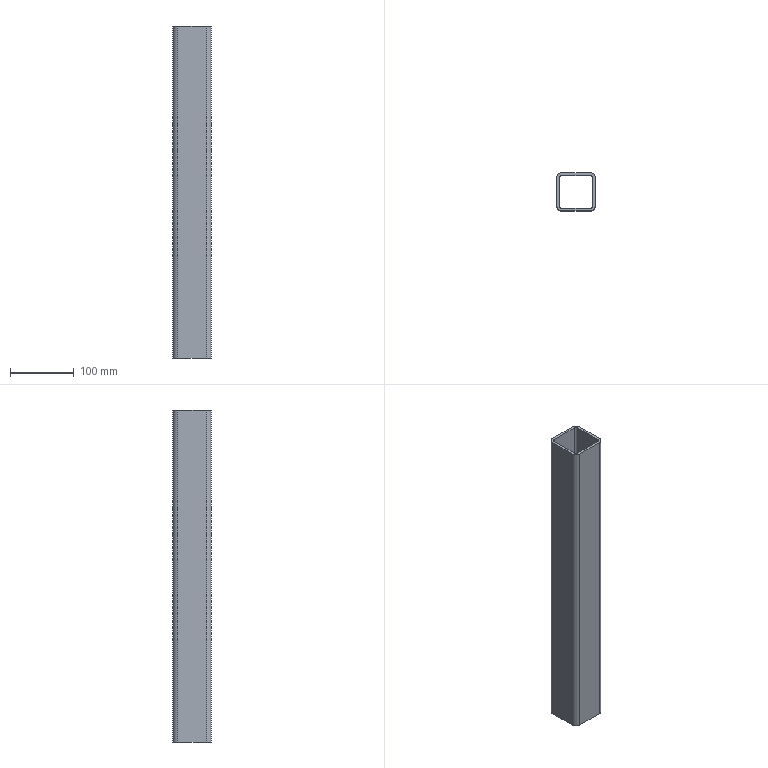Part | SolidWorks | features BaseBody 1 | 1 solid | 18 faces | box 60 x 60 x 520 mm | volume 444494 mm3 | plane 10 | cylinder 8 | commonest cylinder face diameters 8 x4 16 x4
STEP:
#1=CARTESIAN_POINT('',(-130.,44.,-1240.));
#2=VERTEX_POINT('',#1);
#3=CARTESIAN_POINT('',(-130.,44.,-720.));
#4=VERTEX_POINT('',#3);
#5=CARTESIAN_POINT('',(-130.,44.,-1270.));
#6=DIRECTION('',(0.,0.,1.));
#7=VECTOR('',#6,1000.);
#8=LINE('',#5,#7);
#9=EDGE_CURVE('',#2,#4,#8,.T.);
#10=ORIENTED_EDGE('',*,*,#9,.F.);
#11=CARTESIAN_POINT('',(-130.,0.,-1240.));
#12=VERTEX_POINT('',#11);
#13=CARTESIAN_POINT('',(-130.,0.,-1240.));
#14=DIRECTION('',(0.,1.,0.));
#15=VECTOR('',#14,1000.);
#16=LINE('',#13,#15);
#17=EDGE_CURVE('',#12,#2,#16,.T.);
#18=ORIENTED_EDGE('',*,*,#17,.F.);
#19=CARTESIAN_POINT('',(-130.,0.,-720.));
#20=VERTEX_POINT('',#19);
#21=CARTESIAN_POINT('',(-130.,0.,-1270.));
#22=DIRECTION('',(0.,0.,-1.));
#23=VECTOR('',#22,1000.);
#24=LINE('',#21,#23);
#25=EDGE_CURVE('',#20,#12,#24,.T.);
#26=ORIENTED_EDGE('',*,*,#25,.F.);
#27=CARTESIAN_POINT('',(-130.,0.,-720.));
#28=DIRECTION('',(0.,-1.,0.));
#29=VECTOR('',#28,1000.);
#30=LINE('',#27,#29);
#31=EDGE_CURVE('',#4,#20,#30,.T.);
#32=ORIENTED_EDGE('',*,*,#31,.F.);
#33=EDGE_LOOP('',(#10,#18,#26,#32));
#34=FACE_OUTER_BOUND('',#33,.T.);
#35=CARTESIAN_POINT('',(-130.,0.,-1270.));
#36=DIRECTION('',(1.,0.,0.));
#37=DIRECTION('',(0.,0.,-1.));
#38=AXIS2_PLACEMENT_3D('',#35,#36,#37);
#39=PLANE('',#38);
#40=ADVANCED_FACE('',(#34),#39,.F.);
#41=CARTESIAN_POINT('',(-126.,0.,-720.));
#42=VERTEX_POINT('',#41);
#43=CARTESIAN_POINT('',(-122.,-4.,-720.));
#44=VERTEX_POINT('',#43);
#45=CARTESIAN_POINT('',(-122.,0.,-720.));
#46=DIRECTION('',(0.,0.,1.));
#47=DIRECTION('',(1.,0.,0.));
#48=AXIS2_PLACEMENT_3D('',#45,#46,#47);
#49=CIRCLE('',#48,4.);
#50=EDGE_CURVE('',#42,#44,#49,.T.);
#51=ORIENTED_EDGE('',*,*,#50,.F.);
#52=CARTESIAN_POINT('',(-126.,44.,-720.));
#53=VERTEX_POINT('',#52);
#54=CARTESIAN_POINT('',(-126.,1242.,-720.));
#55=DIRECTION('',(0.,-1.,0.));
#56=VECTOR('',#55,1000.);
#57=LINE('',#54,#56);
#58=EDGE_CURVE('',#53,#42,#57,.T.);
#59=ORIENTED_EDGE('',*,*,#58,.F.);
#60=CARTESIAN_POINT('',(-122.,48.,-720.));
#61=VERTEX_POINT('',#60);
#62=CARTESIAN_POINT('',(-122.,44.,-720.));
#63=DIRECTION('',(0.,0.,1.));
#64=DIRECTION('',(1.,0.,0.));
#65=AXIS2_PLACEMENT_3D('',#62,#63,#64);
#66=CIRCLE('',#65,4.);
#67=EDGE_CURVE('',#61,#53,#66,.T.);
#68=ORIENTED_EDGE('',*,*,#67,.F.);
#69=CARTESIAN_POINT('',(-78.,48.,-720.));
#70=VERTEX_POINT('',#69);
#71=CARTESIAN_POINT('',(0.,48.,-720.));
#72=DIRECTION('',(-1.,0.,0.));
#73=VECTOR('',#72,1000.);
#74=LINE('',#71,#73);
#75=EDGE_CURVE('',#70,#61,#74,.T.);
#76=ORIENTED_EDGE('',*,*,#75,.F.);
#77=CARTESIAN_POINT('',(-74.,44.,-720.));
#78=VERTEX_POINT('',#77);
#79=CARTESIAN_POINT('',(-78.,44.,-720.));
#80=DIRECTION('',(0.,0.,1.));
#81=DIRECTION('',(1.,0.,0.));
#82=AXIS2_PLACEMENT_3D('',#79,#80,#81);
#83=CIRCLE('',#82,4.);
#84=EDGE_CURVE('',#78,#70,#83,.T.);
#85=ORIENTED_EDGE('',*,*,#84,.F.);
#86=CARTESIAN_POINT('',(-74.,0.,-720.));
#87=VERTEX_POINT('',#86);
#88=CARTESIAN_POINT('',(-74.,1242.,-720.));
#89=DIRECTION('',(0.,1.,0.));
#90=VECTOR('',#89,1000.);
#91=LINE('',#88,#90);
#92=EDGE_CURVE('',#87,#78,#91,.T.);
#93=ORIENTED_EDGE('',*,*,#92,.F.);
#94=CARTESIAN_POINT('',(-78.,-4.,-720.));
#95=VERTEX_POINT('',#94);
#96=CARTESIAN_POINT('',(-78.,0.,-720.));
#97=DIRECTION('',(0.,0.,1.));
#98=DIRECTION('',(1.,0.,0.));
#99=AXIS2_PLACEMENT_3D('',#96,#97,#98);
#100=CIRCLE('',#99,4.);
#101=EDGE_CURVE('',#95,#87,#100,.T.);
#102=ORIENTED_EDGE('',*,*,#101,.F.);
#103=CARTESIAN_POINT('',(0.,-4.,-720.));
#104=DIRECTION('',(1.,0.,0.));
#105=VECTOR('',#104,1000.);
#106=LINE('',#103,#105);
#107=EDGE_CURVE('',#44,#95,#106,.T.);
#108=ORIENTED_EDGE('',*,*,#107,.F.);
#109=EDGE_LOOP('',(#51,#59,#68,#76,#85,#93,#102,#108));
#110=FACE_BOUND('',#109,.T.);
#111=ORIENTED_EDGE('',*,*,#31,.T.);
#112=CARTESIAN_POINT('',(-122.,-8.,-720.));
#113=VERTEX_POINT('',#112);
#114=CARTESIAN_POINT('',(-122.,0.,-720.));
#115=DIRECTION('',(0.,0.,-1.));
#116=DIRECTION('',(1.,0.,0.));
#117=AXIS2_PLACEMENT_3D('',#114,#115,#116);
#118=CIRCLE('',#117,8.);
#119=EDGE_CURVE('',#113,#20,#118,.T.);
#120=ORIENTED_EDGE('',*,*,#119,.F.);
#121=CARTESIAN_POINT('',(-78.,-8.,-720.));
#122=VERTEX_POINT('',#121);
#123=CARTESIAN_POINT('',(0.,-8.,-720.));
#124=DIRECTION('',(-1.,0.,0.));
#125=VECTOR('',#124,1000.);
#126=LINE('',#123,#125);
#127=EDGE_CURVE('',#122,#113,#126,.T.);
#128=ORIENTED_EDGE('',*,*,#127,.F.);
#129=CARTESIAN_POINT('',(-70.,0.,-720.));
#130=VERTEX_POINT('',#129);
#131=CARTESIAN_POINT('',(-78.,0.,-720.));
#132=DIRECTION('',(0.,0.,-1.));
#133=DIRECTION('',(1.,0.,0.));
#134=AXIS2_PLACEMENT_3D('',#131,#132,#133);
#135=CIRCLE('',#134,8.);
#136=EDGE_CURVE('',#130,#122,#135,.T.);
#137=ORIENTED_EDGE('',*,*,#136,.F.);
#138=CARTESIAN_POINT('',(-70.,44.,-720.));
#139=VERTEX_POINT('',#138);
#140=CARTESIAN_POINT('',(-70.,1242.,-720.));
#141=DIRECTION('',(0.,-1.,0.));
#142=VECTOR('',#141,1000.);
#143=LINE('',#140,#142);
#144=EDGE_CURVE('',#139,#130,#143,.T.);
#145=ORIENTED_EDGE('',*,*,#144,.F.);
#146=CARTESIAN_POINT('',(-78.,52.,-720.));
#147=VERTEX_POINT('',#146);
#148=CARTESIAN_POINT('',(-78.,44.,-720.));
#149=DIRECTION('',(0.,0.,-1.));
#150=DIRECTION('',(1.,0.,0.));
#151=AXIS2_PLACEMENT_3D('',#148,#149,#150);
#152=CIRCLE('',#151,8.);
#153=EDGE_CURVE('',#147,#139,#152,.T.);
#154=ORIENTED_EDGE('',*,*,#153,.F.);
#155=CARTESIAN_POINT('',(-122.,52.,-720.));
#156=VERTEX_POINT('',#155);
#157=CARTESIAN_POINT('',(0.,52.,-720.));
#158=DIRECTION('',(1.,0.,0.));
#159=VECTOR('',#158,1000.);
#160=LINE('',#157,#159);
#161=EDGE_CURVE('',#156,#147,#160,.T.);
#162=ORIENTED_EDGE('',*,*,#161,.F.);
#163=CARTESIAN_POINT('',(-122.,44.,-720.));
#164=DIRECTION('',(0.,0.,-1.));
#165=DIRECTION('',(1.,0.,0.));
#166=AXIS2_PLACEMENT_3D('',#163,#164,#165);
#167=CIRCLE('',#166,8.);
#168=EDGE_CURVE('',#4,#156,#167,.T.);
#169=ORIENTED_EDGE('',*,*,#168,.F.);
#170=EDGE_LOOP('',(#111,#120,#128,#137,#145,#154,#162,#169));
#171=FACE_OUTER_BOUND('',#170,.T.);
#172=CARTESIAN_POINT('',(0.,1242.,-720.));
#173=DIRECTION('',(0.,0.,-1.));
#174=DIRECTION('',(-1.,0.,0.));
#175=AXIS2_PLACEMENT_3D('',#172,#173,#174);
#176=PLANE('',#175);
#177=ADVANCED_FACE('',(#110,#171),#176,.F.);
#178=CARTESIAN_POINT('',(-122.,52.,-1240.));
#179=VERTEX_POINT('',#178);
#180=CARTESIAN_POINT('',(-122.,44.,-1240.));
#181=DIRECTION('',(0.,0.,1.));
#182=DIRECTION('',(1.,0.,0.));
#183=AXIS2_PLACEMENT_3D('',#180,#181,#182);
#184=CIRCLE('',#183,8.);
#185=EDGE_CURVE('',#179,#2,#184,.T.);
#186=ORIENTED_EDGE('',*,*,#185,.T.);
#187=ORIENTED_EDGE('',*,*,#9,.T.);
#188=ORIENTED_EDGE('',*,*,#168,.T.);
#189=CARTESIAN_POINT('',(-122.,52.,-1270.));
#190=DIRECTION('',(0.,0.,-1.));
#191=VECTOR('',#190,1000.);
#192=LINE('',#189,#191);
#193=EDGE_CURVE('',#156,#179,#192,.T.);
#194=ORIENTED_EDGE('',*,*,#193,.T.);
#195=EDGE_LOOP('',(#186,#187,#188,#194));
#196=FACE_OUTER_BOUND('',#195,.T.);
#197=CARTESIAN_POINT('',(-122.,44.,-1270.));
#198=DIRECTION('',(0.,0.,1.));
#199=DIRECTION('',(1.,0.,0.));
#200=AXIS2_PLACEMENT_3D('',#197,#198,#199);
#201=CYLINDRICAL_SURFACE('',#200,8.);
#202=ADVANCED_FACE('',(#196),#201,.T.);
#203=CARTESIAN_POINT('',(-78.,-4.,-1240.));
#204=VERTEX_POINT('',#203);
#205=CARTESIAN_POINT('',(-74.,0.,-1240.));
#206=VERTEX_POINT('',#205);
#207=CARTESIAN_POINT('',(-78.,0.,-1240.));
#208=DIRECTION('',(0.,0.,1.));
#209=DIRECTION('',(1.,0.,0.));
#210=AXIS2_PLACEMENT_3D('',#207,#208,#209);
#211=CIRCLE('',#210,4.);
#212=EDGE_CURVE('',#204,#206,#211,.T.);
#213=ORIENTED_EDGE('',*,*,#212,.T.);
#214=CARTESIAN_POINT('',(-74.,44.,-1240.));
#215=VERTEX_POINT('',#214);
#216=CARTESIAN_POINT('',(-74.,0.,-1240.));
#217=DIRECTION('',(0.,1.,0.));
#218=VECTOR('',#217,1000.);
#219=LINE('',#216,#218);
#220=EDGE_CURVE('',#206,#215,#219,.T.);
#221=ORIENTED_EDGE('',*,*,#220,.T.);
#222=CARTESIAN_POINT('',(-78.,48.,-1240.));
#223=VERTEX_POINT('',#222);
#224=CARTESIAN_POINT('',(-78.,44.,-1240.));
#225=DIRECTION('',(0.,0.,1.));
#226=DIRECTION('',(1.,0.,0.));
#227=AXIS2_PLACEMENT_3D('',#224,#225,#226);
#228=CIRCLE('',#227,4.);
#229=EDGE_CURVE('',#215,#223,#228,.T.);
#230=ORIENTED_EDGE('',*,*,#229,.T.);
#231=CARTESIAN_POINT('',(-122.,48.,-1240.));
#232=VERTEX_POINT('',#231);
#233=CARTESIAN_POINT('',(-670.,48.,-1240.));
#234=DIRECTION('',(-1.,0.,0.));
#235=VECTOR('',#234,1000.);
#236=LINE('',#233,#235);
#237=EDGE_CURVE('',#223,#232,#236,.T.);
#238=ORIENTED_EDGE('',*,*,#237,.T.);
#239=CARTESIAN_POINT('',(-126.,44.,-1240.));
#240=VERTEX_POINT('',#239);
#241=CARTESIAN_POINT('',(-122.,44.,-1240.));
#242=DIRECTION('',(0.,0.,1.));
#243=DIRECTION('',(1.,0.,0.));
#244=AXIS2_PLACEMENT_3D('',#241,#242,#243);
#245=CIRCLE('',#244,4.);
#246=EDGE_CURVE('',#232,#240,#245,.T.);
#247=ORIENTED_EDGE('',*,*,#246,.T.);
#248=CARTESIAN_POINT('',(-126.,0.,-1240.));
#249=VERTEX_POINT('',#248);
#250=CARTESIAN_POINT('',(-126.,0.,-1240.));
#251=DIRECTION('',(0.,-1.,0.));
#252=VECTOR('',#251,1000.);
#253=LINE('',#250,#252);
#254=EDGE_CURVE('',#240,#249,#253,.T.);
#255=ORIENTED_EDGE('',*,*,#254,.T.);
#256=CARTESIAN_POINT('',(-122.,-4.,-1240.));
#257=VERTEX_POINT('',#256);
#258=CARTESIAN_POINT('',(-122.,0.,-1240.));
#259=DIRECTION('',(0.,0.,1.));
#260=DIRECTION('',(1.,0.,0.));
#261=AXIS2_PLACEMENT_3D('',#258,#259,#260);
#262=CIRCLE('',#261,4.);
#263=EDGE_CURVE('',#249,#257,#262,.T.);
#264=ORIENTED_EDGE('',*,*,#263,.T.);
#265=CARTESIAN_POINT('',(-670.,-4.,-1240.));
#266=DIRECTION('',(1.,0.,0.));
#267=VECTOR('',#266,1000.);
#268=LINE('',#265,#267);
#269=EDGE_CURVE('',#257,#204,#268,.T.);
#270=ORIENTED_EDGE('',*,*,#269,.T.);
#271=EDGE_LOOP('',(#213,#221,#230,#238,#247,#255,#264,#270));
#272=FACE_BOUND('',#271,.T.);
#273=CARTESIAN_POINT('',(-78.,52.,-1240.));
#274=VERTEX_POINT('',#273);
#275=CARTESIAN_POINT('',(-670.,52.,-1240.));
#276=DIRECTION('',(1.,0.,0.));
#277=VECTOR('',#276,1000.);
#278=LINE('',#275,#277);
#279=EDGE_CURVE('',#179,#274,#278,.T.);
#280=ORIENTED_EDGE('',*,*,#279,.T.);
#281=CARTESIAN_POINT('',(-70.,44.,-1240.));
#282=VERTEX_POINT('',#281);
#283=CARTESIAN_POINT('',(-78.,44.,-1240.));
#284=DIRECTION('',(0.,0.,-1.));
#285=DIRECTION('',(1.,0.,0.));
#286=AXIS2_PLACEMENT_3D('',#283,#284,#285);
#287=CIRCLE('',#286,8.);
#288=EDGE_CURVE('',#274,#282,#287,.T.);
#289=ORIENTED_EDGE('',*,*,#288,.T.);
#290=CARTESIAN_POINT('',(-70.,0.,-1240.));
#291=VERTEX_POINT('',#290);
#292=CARTESIAN_POINT('',(-70.,0.,-1240.));
#293=DIRECTION('',(0.,-1.,0.));
#294=VECTOR('',#293,1000.);
#295=LINE('',#292,#294);
#296=EDGE_CURVE('',#282,#291,#295,.T.);
#297=ORIENTED_EDGE('',*,*,#296,.T.);
#298=CARTESIAN_POINT('',(-78.,-8.,-1240.));
#299=VERTEX_POINT('',#298);
#300=CARTESIAN_POINT('',(-78.,0.,-1240.));
#301=DIRECTION('',(0.,0.,-1.));
#302=DIRECTION('',(1.,0.,0.));
#303=AXIS2_PLACEMENT_3D('',#300,#301,#302);
#304=CIRCLE('',#303,8.);
#305=EDGE_CURVE('',#291,#299,#304,.T.);
#306=ORIENTED_EDGE('',*,*,#305,.T.);
#307=CARTESIAN_POINT('',(-122.,-8.,-1240.));
#308=VERTEX_POINT('',#307);
#309=CARTESIAN_POINT('',(-670.,-8.,-1240.));
#310=DIRECTION('',(-1.,0.,0.));
#311=VECTOR('',#310,1000.);
#312=LINE('',#309,#311);
#313=EDGE_CURVE('',#299,#308,#312,.T.);
#314=ORIENTED_EDGE('',*,*,#313,.T.);
#315=CARTESIAN_POINT('',(-122.,0.,-1240.));
#316=DIRECTION('',(0.,0.,-1.));
#317=DIRECTION('',(1.,0.,0.));
#318=AXIS2_PLACEMENT_3D('',#315,#316,#317);
#319=CIRCLE('',#318,8.);
#320=EDGE_CURVE('',#308,#12,#319,.T.);
#321=ORIENTED_EDGE('',*,*,#320,.T.);
#322=ORIENTED_EDGE('',*,*,#17,.T.);
#323=ORIENTED_EDGE('',*,*,#185,.F.);
#324=EDGE_LOOP('',(#280,#289,#297,#306,#314,#321,#322,#323));
#325=FACE_OUTER_BOUND('',#324,.T.);
#326=CARTESIAN_POINT('',(-670.,0.,-1240.));
#327=DIRECTION('',(0.,0.,-1.));
#328=DIRECTION('',(-1.,0.,0.));
#329=AXIS2_PLACEMENT_3D('',#326,#327,#328);
#330=PLANE('',#329);
#331=ADVANCED_FACE('',(#272,#325),#330,.T.);
#332=ORIENTED_EDGE('',*,*,#320,.F.);
#333=CARTESIAN_POINT('',(-122.,-8.,-1270.));
#334=DIRECTION('',(0.,0.,1.));
#335=VECTOR('',#334,1000.);
#336=LINE('',#333,#335);
#337=EDGE_CURVE('',#308,#113,#336,.T.);
#338=ORIENTED_EDGE('',*,*,#337,.T.);
#339=ORIENTED_EDGE('',*,*,#119,.T.);
#340=ORIENTED_EDGE('',*,*,#25,.T.);
#341=EDGE_LOOP('',(#332,#338,#339,#340));
#342=FACE_OUTER_BOUND('',#341,.T.);
#343=CARTESIAN_POINT('',(-122.,0.,-1270.));
#344=DIRECTION('',(0.,0.,1.));
#345=DIRECTION('',(1.,0.,0.));
#346=AXIS2_PLACEMENT_3D('',#343,#344,#345);
#347=CYLINDRICAL_SURFACE('',#346,8.);
#348=ADVANCED_FACE('',(#342),#347,.T.);
#349=CARTESIAN_POINT('',(-122.,-4.,-1270.));
#350=DIRECTION('',(0.,0.,1.));
#351=VECTOR('',#350,1000.);
#352=LINE('',#349,#351);
#353=EDGE_CURVE('',#257,#44,#352,.T.);
#354=ORIENTED_EDGE('',*,*,#353,.T.);
#355=ORIENTED_EDGE('',*,*,#107,.T.);
#356=CARTESIAN_POINT('',(-78.,-4.,-1270.));
#357=DIRECTION('',(0.,0.,-1.));
#358=VECTOR('',#357,1000.);
#359=LINE('',#356,#358);
#360=EDGE_CURVE('',#95,#204,#359,.T.);
#361=ORIENTED_EDGE('',*,*,#360,.T.);
#362=ORIENTED_EDGE('',*,*,#269,.F.);
#363=EDGE_LOOP('',(#354,#355,#361,#362));
#364=FACE_OUTER_BOUND('',#363,.T.);
#365=CARTESIAN_POINT('',(-122.,-4.,-1270.));
#366=DIRECTION('',(0.,1.,0.));
#367=DIRECTION('',(0.,0.,1.));
#368=AXIS2_PLACEMENT_3D('',#365,#366,#367);
#369=PLANE('',#368);
#370=ADVANCED_FACE('',(#364),#369,.T.);
#371=ORIENTED_EDGE('',*,*,#263,.F.);
#372=CARTESIAN_POINT('',(-126.,0.,-1270.));
#373=DIRECTION('',(0.,0.,-1.));
#374=VECTOR('',#373,1000.);
#375=LINE('',#372,#374);
#376=EDGE_CURVE('',#42,#249,#375,.T.);
#377=ORIENTED_EDGE('',*,*,#376,.F.);
#378=ORIENTED_EDGE('',*,*,#50,.T.);
#379=ORIENTED_EDGE('',*,*,#353,.F.);
#380=EDGE_LOOP('',(#371,#377,#378,#379));
#381=FACE_OUTER_BOUND('',#380,.T.);
#382=CARTESIAN_POINT('',(-122.,0.,-1270.));
#383=DIRECTION('',(0.,0.,1.));
#384=DIRECTION('',(1.,0.,0.));
#385=AXIS2_PLACEMENT_3D('',#382,#383,#384);
#386=CYLINDRICAL_SURFACE('',#385,4.);
#387=ADVANCED_FACE('',(#381),#386,.F.);
#388=CARTESIAN_POINT('',(-126.,44.,-1270.));
#389=DIRECTION('',(0.,0.,1.));
#390=VECTOR('',#389,1000.);
#391=LINE('',#388,#390);
#392=EDGE_CURVE('',#240,#53,#391,.T.);
#393=ORIENTED_EDGE('',*,*,#392,.T.);
#394=ORIENTED_EDGE('',*,*,#58,.T.);
#395=ORIENTED_EDGE('',*,*,#376,.T.);
#396=ORIENTED_EDGE('',*,*,#254,.F.);
#397=EDGE_LOOP('',(#393,#394,#395,#396));
#398=FACE_OUTER_BOUND('',#397,.T.);
#399=CARTESIAN_POINT('',(-126.,0.,-1270.));
#400=DIRECTION('',(1.,0.,0.));
#401=DIRECTION('',(0.,0.,-1.));
#402=AXIS2_PLACEMENT_3D('',#399,#400,#401);
#403=PLANE('',#402);
#404=ADVANCED_FACE('',(#398),#403,.T.);
#405=ORIENTED_EDGE('',*,*,#246,.F.);
#406=CARTESIAN_POINT('',(-122.,48.,-1270.));
#407=DIRECTION('',(0.,0.,-1.));
#408=VECTOR('',#407,1000.);
#409=LINE('',#406,#408);
#410=EDGE_CURVE('',#61,#232,#409,.T.);
#411=ORIENTED_EDGE('',*,*,#410,.F.);
#412=ORIENTED_EDGE('',*,*,#67,.T.);
#413=ORIENTED_EDGE('',*,*,#392,.F.);
#414=EDGE_LOOP('',(#405,#411,#412,#413));
#415=FACE_OUTER_BOUND('',#414,.T.);
#416=CARTESIAN_POINT('',(-122.,44.,-1270.));
#417=DIRECTION('',(0.,0.,1.));
#418=DIRECTION('',(1.,0.,0.));
#419=AXIS2_PLACEMENT_3D('',#416,#417,#418);
#420=CYLINDRICAL_SURFACE('',#419,4.);
#421=ADVANCED_FACE('',(#415),#420,.F.);
#422=CARTESIAN_POINT('',(-78.,48.,-1270.));
#423=DIRECTION('',(0.,0.,1.));
#424=VECTOR('',#423,1000.);
#425=LINE('',#422,#424);
#426=EDGE_CURVE('',#223,#70,#425,.T.);
#427=ORIENTED_EDGE('',*,*,#426,.T.);
#428=ORIENTED_EDGE('',*,*,#75,.T.);
#429=ORIENTED_EDGE('',*,*,#410,.T.);
#430=ORIENTED_EDGE('',*,*,#237,.F.);
#431=EDGE_LOOP('',(#427,#428,#429,#430));
#432=FACE_OUTER_BOUND('',#431,.T.);
#433=CARTESIAN_POINT('',(-78.,48.,-1270.));
#434=DIRECTION('',(0.,-1.,0.));
#435=DIRECTION('',(0.,0.,-1.));
#436=AXIS2_PLACEMENT_3D('',#433,#434,#435);
#437=PLANE('',#436);
#438=ADVANCED_FACE('',(#432),#437,.T.);
#439=ORIENTED_EDGE('',*,*,#229,.F.);
#440=CARTESIAN_POINT('',(-74.,44.,-1270.));
#441=DIRECTION('',(0.,0.,-1.));
#442=VECTOR('',#441,1000.);
#443=LINE('',#440,#442);
#444=EDGE_CURVE('',#78,#215,#443,.T.);
#445=ORIENTED_EDGE('',*,*,#444,.F.);
#446=ORIENTED_EDGE('',*,*,#84,.T.);
#447=ORIENTED_EDGE('',*,*,#426,.F.);
#448=EDGE_LOOP('',(#439,#445,#446,#447));
#449=FACE_OUTER_BOUND('',#448,.T.);
#450=CARTESIAN_POINT('',(-78.,44.,-1270.));
#451=DIRECTION('',(0.,0.,1.));
#452=DIRECTION('',(1.,0.,0.));
#453=AXIS2_PLACEMENT_3D('',#450,#451,#452);
#454=CYLINDRICAL_SURFACE('',#453,4.);
#455=ADVANCED_FACE('',(#449),#454,.F.);
#456=CARTESIAN_POINT('',(-74.,0.,-1270.));
#457=DIRECTION('',(0.,0.,1.));
#458=VECTOR('',#457,1000.);
#459=LINE('',#456,#458);
#460=EDGE_CURVE('',#206,#87,#459,.T.);
#461=ORIENTED_EDGE('',*,*,#460,.T.);
#462=ORIENTED_EDGE('',*,*,#92,.T.);
#463=ORIENTED_EDGE('',*,*,#444,.T.);
#464=ORIENTED_EDGE('',*,*,#220,.F.);
#465=EDGE_LOOP('',(#461,#462,#463,#464));
#466=FACE_OUTER_BOUND('',#465,.T.);
#467=CARTESIAN_POINT('',(-74.,44.,-1270.));
#468=DIRECTION('',(-1.,0.,0.));
#469=DIRECTION('',(0.,0.,1.));
#470=AXIS2_PLACEMENT_3D('',#467,#468,#469);
#471=PLANE('',#470);
#472=ADVANCED_FACE('',(#466),#471,.T.);
#473=ORIENTED_EDGE('',*,*,#212,.F.);
#474=ORIENTED_EDGE('',*,*,#360,.F.);
#475=ORIENTED_EDGE('',*,*,#101,.T.);
#476=ORIENTED_EDGE('',*,*,#460,.F.);
#477=EDGE_LOOP('',(#473,#474,#475,#476));
#478=FACE_OUTER_BOUND('',#477,.T.);
#479=CARTESIAN_POINT('',(-78.,0.,-1270.));
#480=DIRECTION('',(0.,0.,1.));
#481=DIRECTION('',(1.,0.,0.));
#482=AXIS2_PLACEMENT_3D('',#479,#480,#481);
#483=CYLINDRICAL_SURFACE('',#482,4.);
#484=ADVANCED_FACE('',(#478),#483,.F.);
#485=ORIENTED_EDGE('',*,*,#337,.F.);
#486=ORIENTED_EDGE('',*,*,#313,.F.);
#487=CARTESIAN_POINT('',(-78.,-8.,-1270.));
#488=DIRECTION('',(0.,0.,-1.));
#489=VECTOR('',#488,1000.);
#490=LINE('',#487,#489);
#491=EDGE_CURVE('',#122,#299,#490,.T.);
#492=ORIENTED_EDGE('',*,*,#491,.F.);
#493=ORIENTED_EDGE('',*,*,#127,.T.);
#494=EDGE_LOOP('',(#485,#486,#492,#493));
#495=FACE_OUTER_BOUND('',#494,.T.);
#496=CARTESIAN_POINT('',(-122.,-8.,-1270.));
#497=DIRECTION('',(0.,1.,0.));
#498=DIRECTION('',(0.,0.,1.));
#499=AXIS2_PLACEMENT_3D('',#496,#497,#498);
#500=PLANE('',#499);
#501=ADVANCED_FACE('',(#495),#500,.F.);
#502=ORIENTED_EDGE('',*,*,#305,.F.);
#503=CARTESIAN_POINT('',(-70.,0.,-1270.));
#504=DIRECTION('',(0.,0.,1.));
#505=VECTOR('',#504,1000.);
#506=LINE('',#503,#505);
#507=EDGE_CURVE('',#291,#130,#506,.T.);
#508=ORIENTED_EDGE('',*,*,#507,.T.);
#509=ORIENTED_EDGE('',*,*,#136,.T.);
#510=ORIENTED_EDGE('',*,*,#491,.T.);
#511=EDGE_LOOP('',(#502,#508,#509,#510));
#512=FACE_OUTER_BOUND('',#511,.T.);
#513=CARTESIAN_POINT('',(-78.,0.,-1270.));
#514=DIRECTION('',(0.,0.,1.));
#515=DIRECTION('',(1.,0.,0.));
#516=AXIS2_PLACEMENT_3D('',#513,#514,#515);
#517=CYLINDRICAL_SURFACE('',#516,8.);
#518=ADVANCED_FACE('',(#512),#517,.T.);
#519=ORIENTED_EDGE('',*,*,#507,.F.);
#520=ORIENTED_EDGE('',*,*,#296,.F.);
#521=CARTESIAN_POINT('',(-70.,44.,-1270.));
#522=DIRECTION('',(0.,0.,-1.));
#523=VECTOR('',#522,1000.);
#524=LINE('',#521,#523);
#525=EDGE_CURVE('',#139,#282,#524,.T.);
#526=ORIENTED_EDGE('',*,*,#525,.F.);
#527=ORIENTED_EDGE('',*,*,#144,.T.);
#528=EDGE_LOOP('',(#519,#520,#526,#527));
#529=FACE_OUTER_BOUND('',#528,.T.);
#530=CARTESIAN_POINT('',(-70.,44.,-1270.));
#531=DIRECTION('',(-1.,0.,0.));
#532=DIRECTION('',(0.,0.,1.));
#533=AXIS2_PLACEMENT_3D('',#530,#531,#532);
#534=PLANE('',#533);
#535=ADVANCED_FACE('',(#529),#534,.F.);
#536=ORIENTED_EDGE('',*,*,#288,.F.);
#537=CARTESIAN_POINT('',(-78.,52.,-1270.));
#538=DIRECTION('',(0.,0.,1.));
#539=VECTOR('',#538,1000.);
#540=LINE('',#537,#539);
#541=EDGE_CURVE('',#274,#147,#540,.T.);
#542=ORIENTED_EDGE('',*,*,#541,.T.);
#543=ORIENTED_EDGE('',*,*,#153,.T.);
#544=ORIENTED_EDGE('',*,*,#525,.T.);
#545=EDGE_LOOP('',(#536,#542,#543,#544));
#546=FACE_OUTER_BOUND('',#545,.T.);
#547=CARTESIAN_POINT('',(-78.,44.,-1270.));
#548=DIRECTION('',(0.,0.,1.));
#549=DIRECTION('',(1.,0.,0.));
#550=AXIS2_PLACEMENT_3D('',#547,#548,#549);
#551=CYLINDRICAL_SURFACE('',#550,8.);
#552=ADVANCED_FACE('',(#546),#551,.T.);
#553=ORIENTED_EDGE('',*,*,#541,.F.);
#554=ORIENTED_EDGE('',*,*,#279,.F.);
#555=ORIENTED_EDGE('',*,*,#193,.F.);
#556=ORIENTED_EDGE('',*,*,#161,.T.);
#557=EDGE_LOOP('',(#553,#554,#555,#556));
#558=FACE_OUTER_BOUND('',#557,.T.);
#559=CARTESIAN_POINT('',(-78.,52.,-1270.));
#560=DIRECTION('',(0.,-1.,0.));
#561=DIRECTION('',(0.,0.,-1.));
#562=AXIS2_PLACEMENT_3D('',#559,#560,#561);
#563=PLANE('',#562);
#564=ADVANCED_FACE('',(#558),#563,.F.);
#565=CLOSED_SHELL('',(#40,#177,#202,#331,#348,#370,#387,#404,#421,#438,#455,#472,#484,#501,#518,#535,#552,#564));
#566=MANIFOLD_SOLID_BREP('',#565);
#567=CARTESIAN_POINT('',(0.,0.,0.));
#568=DIRECTION('',(0.,0.,1.));
#569=DIRECTION('',(1.,0.,0.));
#570=AXIS2_PLACEMENT_3D('',#567,#568,#569);
#571=(LENGTH_UNIT()NAMED_UNIT(*)SI_UNIT(.MILLI.,.METRE.));
#572=UNCERTAINTY_MEASURE_WITH_UNIT(LENGTH_MEASURE(0.00001),#571,'','');
#573=(NAMED_UNIT(*)PLANE_ANGLE_UNIT()SI_UNIT($,.RADIAN.));
#574=(NAMED_UNIT(*)SI_UNIT($,.STERADIAN.)SOLID_ANGLE_UNIT());
#575=(GEOMETRIC_REPRESENTATION_CONTEXT(3)GLOBAL_UNCERTAINTY_ASSIGNED_CONTEXT((#572))GLOBAL_UNIT_ASSIGNED_CONTEXT((#571,#573,#574))REPRESENTATION_CONTEXT('',''));
#576=ADVANCED_BREP_SHAPE_REPRESENTATION('',(#566,#570),#575);